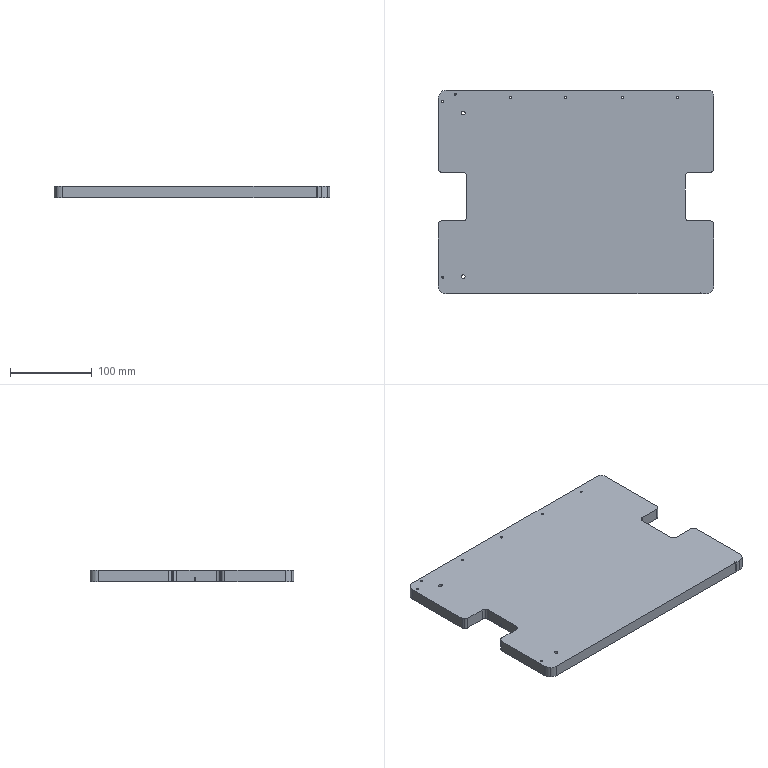Part | STEP file | ASND-0110-PWP TOP tu pang 20130814.sldasm-Part-2aq | 1 solid | 76 faces | box 337.093 x 249.456 x 14.1 mm | volume 1124942 mm3 | cylinder 54 | plane 22 | commonest cylinder face diameters 10 x16 2.5 x14 3 x6 9 x6 20 x6 4.5 x4